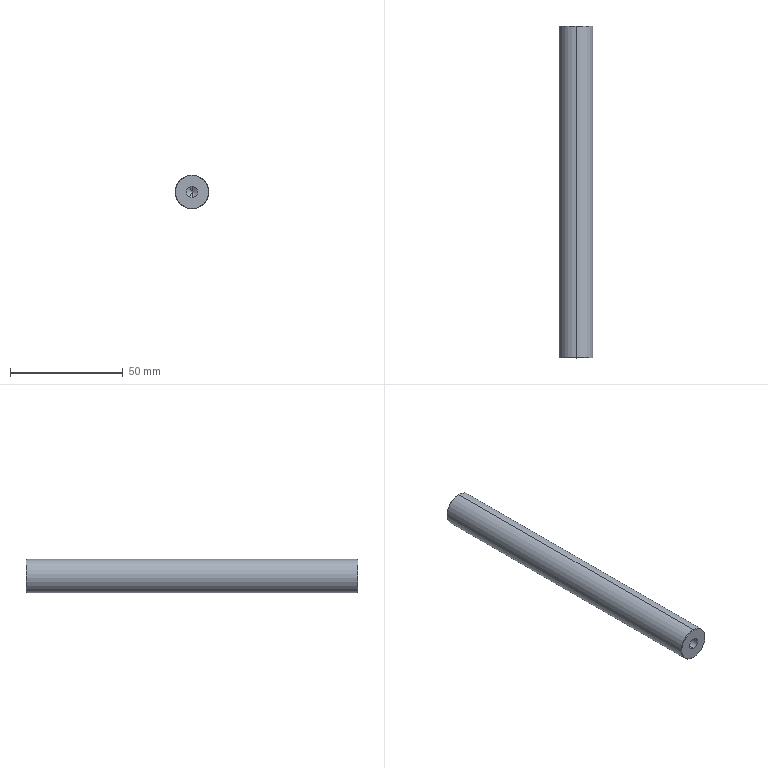Part | STEP file | 1 solid | 16 faces | box 15 x 147 x 15 mm | volume 25052 mm3 | cone 8 | cylinder 6 | plane 2 | commonest cylinder face diameters 5 x4 15 x2
STEP:
#1=CARTESIAN_POINT('',(0.,0.,0.));
#2=DIRECTION('',(0.,0.,1.));
#3=DIRECTION('',(1.,0.,0.));
#4=AXIS2_PLACEMENT_3D('',#1,#2,#3);
#5=CARTESIAN_POINT('',(0.,-73.5,-7.3));
#6=VERTEX_POINT('',#5);
#7=CARTESIAN_POINT('',(0.,-73.5,7.3));
#8=VERTEX_POINT('',#7);
#9=CARTESIAN_POINT('',(0.,-73.5,0.));
#10=DIRECTION('',(0.,-1.,0.));
#11=DIRECTION('',(0.,0.,1.));
#12=AXIS2_PLACEMENT_3D('',#9,#10,#11);
#13=CIRCLE('',#12,7.3);
#14=CARTESIAN_POINT('',(0.,-73.3,0.));
#15=DIRECTION('',(0.,1.,0.));
#16=DIRECTION('',(0.,0.,1.));
#17=AXIS2_PLACEMENT_3D('',#14,#15,#16);
#18=CONICAL_SURFACE('',#17,7.5,0.7854);
#19=CARTESIAN_POINT('',(6.283,-0.2));
#20=DIRECTION('',(-1.,0.));
#21=VECTOR('',#20,1.);
#22=LINE('',#19,#21);
#23=(GEOMETRIC_REPRESENTATION_CONTEXT(2)PARAMETRIC_REPRESENTATION_CONTEXT()REPRESENTATION_CONTEXT('',''));
#24=DEFINITIONAL_REPRESENTATION('',(#22),#23);
#25=PCURVE('',#18,#24);
#26=CARTESIAN_POINT('',(0.,-73.5,0.));
#27=DIRECTION('',(0.,1.,0.));
#28=DIRECTION('',(0.,0.,1.));
#29=AXIS2_PLACEMENT_3D('',#26,#27,#28);
#30=PLANE('',#29);
#31=CARTESIAN_POINT('',(7.3,0.));
#32=CARTESIAN_POINT('',(7.3,-12.644));
#33=CARTESIAN_POINT('',(-3.65,-6.322));
#34=CARTESIAN_POINT('',(-14.6,0.));
#35=CARTESIAN_POINT('',(-3.65,6.322));
#36=CARTESIAN_POINT('',(7.3,12.644));
#37=CARTESIAN_POINT('',(7.3,0.));
#38=(BOUNDED_CURVE()B_SPLINE_CURVE(2,(#31,#32,#33,#34,#35,#36,#37),.UNSPECIFIED.,.T.,.F.)B_SPLINE_CURVE_WITH_KNOTS((1,2,2,2,2,1),(-2.094,0.,2.094,4.189,6.283,8.378),.UNSPECIFIED.)CURVE()GEOMETRIC_REPRESENTATION_ITEM()RATIONAL_B_SPLINE_CURVE((1.,0.5,1.,0.5,1.,0.5,1.))REPRESENTATION_ITEM(''));
#39=(GEOMETRIC_REPRESENTATION_CONTEXT(2)PARAMETRIC_REPRESENTATION_CONTEXT()REPRESENTATION_CONTEXT('',''));
#40=DEFINITIONAL_REPRESENTATION('',(#38),#39);
#41=PCURVE('',#30,#40);
#42=SURFACE_CURVE('',#13,(#25,#41),.PCURVE_S1.);
#43=EDGE_CURVE('',#6,#8,#42,.T.);
#44=ORIENTED_EDGE('',*,*,#43,.F.);
#45=CARTESIAN_POINT('',(0.,-73.3,-7.5));
#46=VERTEX_POINT('',#45);
#47=CARTESIAN_POINT('',(0.,-73.3,-7.5));
#48=DIRECTION('',(0.,0.7071,-0.7071));
#49=VECTOR('',#48,1.);
#50=LINE('',#47,#49);
#51=CARTESIAN_POINT('',(3.142,0.));
#52=DIRECTION('',(0.,1.));
#53=VECTOR('',#52,1.);
#54=LINE('',#51,#53);
#55=(GEOMETRIC_REPRESENTATION_CONTEXT(2)PARAMETRIC_REPRESENTATION_CONTEXT()REPRESENTATION_CONTEXT('',''));
#56=DEFINITIONAL_REPRESENTATION('',(#54),#55);
#57=PCURVE('',#18,#56);
#58=CARTESIAN_POINT('',(0.,-73.3,0.));
#59=DIRECTION('',(0.,1.,0.));
#60=DIRECTION('',(0.,0.,1.));
#61=AXIS2_PLACEMENT_3D('',#58,#59,#60);
#62=CONICAL_SURFACE('',#61,7.5,0.7854);
#63=CARTESIAN_POINT('',(3.142,0.));
#64=DIRECTION('',(0.,1.));
#65=VECTOR('',#64,1.);
#66=LINE('',#63,#65);
#67=(GEOMETRIC_REPRESENTATION_CONTEXT(2)PARAMETRIC_REPRESENTATION_CONTEXT()REPRESENTATION_CONTEXT('',''));
#68=DEFINITIONAL_REPRESENTATION('',(#66),#67);
#69=PCURVE('',#62,#68);
#70=SURFACE_CURVE('',#50,(#57,#69),.PCURVE_S1.);
#71=EDGE_CURVE('',#6,#46,#70,.T.);
#72=ORIENTED_EDGE('',*,*,#71,.T.);
#73=CARTESIAN_POINT('',(0.,-73.3,7.5));
#74=VERTEX_POINT('',#73);
#75=CARTESIAN_POINT('',(0.,-73.3,0.));
#76=DIRECTION('',(0.,1.,0.));
#77=DIRECTION('',(0.,0.,1.));
#78=AXIS2_PLACEMENT_3D('',#75,#76,#77);
#79=CIRCLE('',#78,7.5);
#80=CARTESIAN_POINT('',(0.,0.));
#81=DIRECTION('',(1.,0.));
#82=VECTOR('',#81,1.);
#83=LINE('',#80,#82);
#84=(GEOMETRIC_REPRESENTATION_CONTEXT(2)PARAMETRIC_REPRESENTATION_CONTEXT()REPRESENTATION_CONTEXT('',''));
#85=DEFINITIONAL_REPRESENTATION('',(#83),#84);
#86=PCURVE('',#18,#85);
#87=CARTESIAN_POINT('',(0.,73.5,0.));
#88=DIRECTION('',(0.,-1.,0.));
#89=DIRECTION('',(0.,0.,-1.));
#90=AXIS2_PLACEMENT_3D('',#87,#88,#89);
#91=CYLINDRICAL_SURFACE('',#90,7.5);
#92=CARTESIAN_POINT('',(3.142,146.8));
#93=DIRECTION('',(-1.,0.));
#94=VECTOR('',#93,1.);
#95=LINE('',#92,#94);
#96=(GEOMETRIC_REPRESENTATION_CONTEXT(2)PARAMETRIC_REPRESENTATION_CONTEXT()REPRESENTATION_CONTEXT('',''));
#97=DEFINITIONAL_REPRESENTATION('',(#95),#96);
#98=PCURVE('',#91,#97);
#99=SURFACE_CURVE('',#79,(#86,#98),.PCURVE_S1.);
#100=EDGE_CURVE('',#74,#46,#99,.T.);
#101=ORIENTED_EDGE('',*,*,#100,.F.);
#102=CARTESIAN_POINT('',(0.,-73.3,7.5));
#103=DIRECTION('',(0.,0.7071,0.7071));
#104=VECTOR('',#103,1.);
#105=LINE('',#102,#104);
#106=CARTESIAN_POINT('',(0.,0.));
#107=DIRECTION('',(0.,1.));
#108=VECTOR('',#107,1.);
#109=LINE('',#106,#108);
#110=(GEOMETRIC_REPRESENTATION_CONTEXT(2)PARAMETRIC_REPRESENTATION_CONTEXT()REPRESENTATION_CONTEXT('',''));
#111=DEFINITIONAL_REPRESENTATION('',(#109),#110);
#112=PCURVE('',#18,#111);
#113=CARTESIAN_POINT('',(6.283,0.));
#114=DIRECTION('',(0.,1.));
#115=VECTOR('',#114,1.);
#116=LINE('',#113,#115);
#117=(GEOMETRIC_REPRESENTATION_CONTEXT(2)PARAMETRIC_REPRESENTATION_CONTEXT()REPRESENTATION_CONTEXT('',''));
#118=DEFINITIONAL_REPRESENTATION('',(#116),#117);
#119=PCURVE('',#62,#118);
#120=SURFACE_CURVE('',#105,(#112,#119),.PCURVE_S1.);
#121=EDGE_CURVE('',#8,#74,#120,.T.);
#122=ORIENTED_EDGE('',*,*,#121,.F.);
#123=EDGE_LOOP('',(#44,#72,#101,#122));
#124=FACE_BOUND('',#123,.T.);
#125=ADVANCED_FACE('',(#124),#18,.T.);
#126=CARTESIAN_POINT('',(0.,73.5,7.3));
#127=VERTEX_POINT('',#126);
#128=CARTESIAN_POINT('',(0.,73.5,-7.3));
#129=VERTEX_POINT('',#128);
#130=CARTESIAN_POINT('',(0.,73.5,0.));
#131=DIRECTION('',(0.,1.,0.));
#132=DIRECTION('',(0.,0.,1.));
#133=AXIS2_PLACEMENT_3D('',#130,#131,#132);
#134=CIRCLE('',#133,7.3);
#135=CARTESIAN_POINT('',(0.,73.5,0.));
#136=DIRECTION('',(0.,-1.,0.));
#137=DIRECTION('',(0.,0.,-1.));
#138=AXIS2_PLACEMENT_3D('',#135,#136,#137);
#139=CONICAL_SURFACE('',#138,7.3,0.7854);
#140=CARTESIAN_POINT('',(3.142,0.));
#141=DIRECTION('',(-1.,0.));
#142=VECTOR('',#141,1.);
#143=LINE('',#140,#142);
#144=(GEOMETRIC_REPRESENTATION_CONTEXT(2)PARAMETRIC_REPRESENTATION_CONTEXT()REPRESENTATION_CONTEXT('',''));
#145=DEFINITIONAL_REPRESENTATION('',(#143),#144);
#146=PCURVE('',#139,#145);
#147=CARTESIAN_POINT('',(0.,73.5,0.));
#148=DIRECTION('',(0.,1.,0.));
#149=DIRECTION('',(0.,0.,1.));
#150=AXIS2_PLACEMENT_3D('',#147,#148,#149);
#151=PLANE('',#150);
#152=CARTESIAN_POINT('',(0.,0.));
#153=DIRECTION('',(1.,0.));
#154=AXIS2_PLACEMENT_2D('',#152,#153);
#155=CIRCLE('',#154,7.3);
#156=(GEOMETRIC_REPRESENTATION_CONTEXT(2)PARAMETRIC_REPRESENTATION_CONTEXT()REPRESENTATION_CONTEXT('',''));
#157=DEFINITIONAL_REPRESENTATION('',(#155),#156);
#158=PCURVE('',#151,#157);
#159=SURFACE_CURVE('',#134,(#146,#158),.PCURVE_S1.);
#160=EDGE_CURVE('',#127,#129,#159,.T.);
#161=ORIENTED_EDGE('',*,*,#160,.F.);
#162=CARTESIAN_POINT('',(0.,73.3,7.5));
#163=VERTEX_POINT('',#162);
#164=CARTESIAN_POINT('',(0.,73.5,7.3));
#165=DIRECTION('',(0.,-0.7071,0.7071));
#166=VECTOR('',#165,1.);
#167=LINE('',#164,#166);
#168=CARTESIAN_POINT('',(3.142,0.));
#169=DIRECTION('',(0.,1.));
#170=VECTOR('',#169,1.);
#171=LINE('',#168,#170);
#172=(GEOMETRIC_REPRESENTATION_CONTEXT(2)PARAMETRIC_REPRESENTATION_CONTEXT()REPRESENTATION_CONTEXT('',''));
#173=DEFINITIONAL_REPRESENTATION('',(#171),#172);
#174=PCURVE('',#139,#173);
#175=CARTESIAN_POINT('',(0.,73.5,0.));
#176=DIRECTION('',(0.,-1.,0.));
#177=DIRECTION('',(0.,0.,-1.));
#178=AXIS2_PLACEMENT_3D('',#175,#176,#177);
#179=CONICAL_SURFACE('',#178,7.3,0.7854);
#180=CARTESIAN_POINT('',(3.142,0.));
#181=DIRECTION('',(0.,1.));
#182=VECTOR('',#181,1.);
#183=LINE('',#180,#182);
#184=(GEOMETRIC_REPRESENTATION_CONTEXT(2)PARAMETRIC_REPRESENTATION_CONTEXT()REPRESENTATION_CONTEXT('',''));
#185=DEFINITIONAL_REPRESENTATION('',(#183),#184);
#186=PCURVE('',#179,#185);
#187=SURFACE_CURVE('',#167,(#174,#186),.PCURVE_S1.);
#188=EDGE_CURVE('',#127,#163,#187,.T.);
#189=ORIENTED_EDGE('',*,*,#188,.T.);
#190=CARTESIAN_POINT('',(0.,73.3,-7.5));
#191=VERTEX_POINT('',#190);
#192=CARTESIAN_POINT('',(0.,73.3,0.));
#193=DIRECTION('',(0.,-1.,0.));
#194=DIRECTION('',(0.,0.,1.));
#195=AXIS2_PLACEMENT_3D('',#192,#193,#194);
#196=CIRCLE('',#195,7.5);
#197=CARTESIAN_POINT('',(-3.142,0.2));
#198=DIRECTION('',(1.,0.));
#199=VECTOR('',#198,1.);
#200=LINE('',#197,#199);
#201=(GEOMETRIC_REPRESENTATION_CONTEXT(2)PARAMETRIC_REPRESENTATION_CONTEXT()REPRESENTATION_CONTEXT('',''));
#202=DEFINITIONAL_REPRESENTATION('',(#200),#201);
#203=PCURVE('',#139,#202);
#204=CARTESIAN_POINT('',(-3.142,0.2));
#205=DIRECTION('',(1.,0.));
#206=VECTOR('',#205,1.);
#207=LINE('',#204,#206);
#208=(GEOMETRIC_REPRESENTATION_CONTEXT(2)PARAMETRIC_REPRESENTATION_CONTEXT()REPRESENTATION_CONTEXT('',''));
#209=DEFINITIONAL_REPRESENTATION('',(#207),#208);
#210=PCURVE('',#91,#209);
#211=SURFACE_CURVE('',#196,(#203,#210),.PCURVE_S1.);
#212=EDGE_CURVE('',#191,#163,#211,.T.);
#213=ORIENTED_EDGE('',*,*,#212,.F.);
#214=CARTESIAN_POINT('',(0.,73.5,-7.3));
#215=DIRECTION('',(0.,-0.7071,-0.7071));
#216=VECTOR('',#215,1.);
#217=LINE('',#214,#216);
#218=CARTESIAN_POINT('',(0.,0.));
#219=DIRECTION('',(0.,1.));
#220=VECTOR('',#219,1.);
#221=LINE('',#218,#220);
#222=(GEOMETRIC_REPRESENTATION_CONTEXT(2)PARAMETRIC_REPRESENTATION_CONTEXT()REPRESENTATION_CONTEXT('',''));
#223=DEFINITIONAL_REPRESENTATION('',(#221),#222);
#224=PCURVE('',#139,#223);
#225=CARTESIAN_POINT('',(6.283,0.));
#226=DIRECTION('',(0.,1.));
#227=VECTOR('',#226,1.);
#228=LINE('',#225,#227);
#229=(GEOMETRIC_REPRESENTATION_CONTEXT(2)PARAMETRIC_REPRESENTATION_CONTEXT()REPRESENTATION_CONTEXT('',''));
#230=DEFINITIONAL_REPRESENTATION('',(#228),#229);
#231=PCURVE('',#179,#230);
#232=SURFACE_CURVE('',#217,(#224,#231),.PCURVE_S1.);
#233=EDGE_CURVE('',#129,#191,#232,.T.);
#234=ORIENTED_EDGE('',*,*,#233,.F.);
#235=EDGE_LOOP('',(#161,#189,#213,#234));
#236=FACE_BOUND('',#235,.T.);
#237=ADVANCED_FACE('',(#236),#139,.T.);
#238=CARTESIAN_POINT('',(0.,-50.5,-2.5));
#239=VERTEX_POINT('',#238);
#240=CARTESIAN_POINT('',(0.,-73.5,-2.5));
#241=VERTEX_POINT('',#240);
#242=CARTESIAN_POINT('',(0.,-73.5,-2.5));
#243=DIRECTION('',(0.,-1.,0.));
#244=VECTOR('',#243,1.);
#245=LINE('',#242,#244);
#246=CARTESIAN_POINT('',(0.,-73.5,0.));
#247=DIRECTION('',(0.,-1.,0.));
#248=DIRECTION('',(0.,0.,-1.));
#249=AXIS2_PLACEMENT_3D('',#246,#247,#248);
#250=CYLINDRICAL_SURFACE('',#249,2.5);
#251=CARTESIAN_POINT('',(6.283,0.));
#252=DIRECTION('',(0.,1.));
#253=VECTOR('',#252,1.);
#254=LINE('',#251,#253);
#255=(GEOMETRIC_REPRESENTATION_CONTEXT(2)PARAMETRIC_REPRESENTATION_CONTEXT()REPRESENTATION_CONTEXT('',''));
#256=DEFINITIONAL_REPRESENTATION('',(#254),#255);
#257=PCURVE('',#250,#256);
#258=CARTESIAN_POINT('',(0.,-73.5,0.));
#259=DIRECTION('',(0.,-1.,0.));
#260=DIRECTION('',(0.,0.,-1.));
#261=AXIS2_PLACEMENT_3D('',#258,#259,#260);
#262=CYLINDRICAL_SURFACE('',#261,2.5);
#263=CARTESIAN_POINT('',(0.,0.));
#264=DIRECTION('',(0.,1.));
#265=VECTOR('',#264,1.);
#266=LINE('',#263,#265);
#267=(GEOMETRIC_REPRESENTATION_CONTEXT(2)PARAMETRIC_REPRESENTATION_CONTEXT()REPRESENTATION_CONTEXT('',''));
#268=DEFINITIONAL_REPRESENTATION('',(#266),#267);
#269=PCURVE('',#262,#268);
#270=SURFACE_CURVE('',#245,(#257,#269),.PCURVE_S1.);
#271=EDGE_CURVE('',#239,#241,#270,.T.);
#272=ORIENTED_EDGE('',*,*,#271,.T.);
#273=CARTESIAN_POINT('',(0.,-73.5,2.5));
#274=VERTEX_POINT('',#273);
#275=CARTESIAN_POINT('',(0.,-73.5,0.));
#276=DIRECTION('',(0.,-1.,0.));
#277=DIRECTION('',(0.,0.,-1.));
#278=AXIS2_PLACEMENT_3D('',#275,#276,#277);
#279=CIRCLE('',#278,2.5);
#280=CARTESIAN_POINT('',(0.,0.));
#281=DIRECTION('',(1.,0.));
#282=VECTOR('',#281,1.);
#283=LINE('',#280,#282);
#284=(GEOMETRIC_REPRESENTATION_CONTEXT(2)PARAMETRIC_REPRESENTATION_CONTEXT()REPRESENTATION_CONTEXT('',''));
#285=DEFINITIONAL_REPRESENTATION('',(#283),#284);
#286=PCURVE('',#250,#285);
#287=CARTESIAN_POINT('',(-2.5,0.));
#288=CARTESIAN_POINT('',(-2.5,4.33));
#289=CARTESIAN_POINT('',(1.25,2.165));
#290=CARTESIAN_POINT('',(5.,0.));
#291=CARTESIAN_POINT('',(1.25,-2.165));
#292=CARTESIAN_POINT('',(-2.5,-4.33));
#293=CARTESIAN_POINT('',(-2.5,0.));
#294=(BOUNDED_CURVE()B_SPLINE_CURVE(2,(#287,#288,#289,#290,#291,#292,#293),.UNSPECIFIED.,.T.,.F.)B_SPLINE_CURVE_WITH_KNOTS((1,2,2,2,2,1),(-2.094,0.,2.094,4.189,6.283,8.378),.UNSPECIFIED.)CURVE()GEOMETRIC_REPRESENTATION_ITEM()RATIONAL_B_SPLINE_CURVE((1.,0.5,1.,0.5,1.,0.5,1.))REPRESENTATION_ITEM(''));
#295=(GEOMETRIC_REPRESENTATION_CONTEXT(2)PARAMETRIC_REPRESENTATION_CONTEXT()REPRESENTATION_CONTEXT('',''));
#296=DEFINITIONAL_REPRESENTATION('',(#294),#295);
#297=PCURVE('',#30,#296);
#298=SURFACE_CURVE('',#279,(#286,#297),.PCURVE_S1.);
#299=EDGE_CURVE('',#274,#241,#298,.T.);
#300=ORIENTED_EDGE('',*,*,#299,.F.);
#301=CARTESIAN_POINT('',(0.,-50.5,2.5));
#302=VERTEX_POINT('',#301);
#303=CARTESIAN_POINT('',(0.,-73.5,2.5));
#304=DIRECTION('',(0.,-1.,0.));
#305=VECTOR('',#304,1.);
#306=LINE('',#303,#305);
#307=CARTESIAN_POINT('',(3.142,0.));
#308=DIRECTION('',(0.,1.));
#309=VECTOR('',#308,1.);
#310=LINE('',#307,#309);
#311=(GEOMETRIC_REPRESENTATION_CONTEXT(2)PARAMETRIC_REPRESENTATION_CONTEXT()REPRESENTATION_CONTEXT('',''));
#312=DEFINITIONAL_REPRESENTATION('',(#310),#311);
#313=PCURVE('',#250,#312);
#314=CARTESIAN_POINT('',(3.142,0.));
#315=DIRECTION('',(0.,1.));
#316=VECTOR('',#315,1.);
#317=LINE('',#314,#316);
#318=(GEOMETRIC_REPRESENTATION_CONTEXT(2)PARAMETRIC_REPRESENTATION_CONTEXT()REPRESENTATION_CONTEXT('',''));
#319=DEFINITIONAL_REPRESENTATION('',(#317),#318);
#320=PCURVE('',#262,#319);
#321=SURFACE_CURVE('',#306,(#313,#320),.PCURVE_S1.);
#322=EDGE_CURVE('',#302,#274,#321,.T.);
#323=ORIENTED_EDGE('',*,*,#322,.F.);
#324=CARTESIAN_POINT('',(0.,-50.5,0.));
#325=DIRECTION('',(0.,-1.,0.));
#326=DIRECTION('',(0.,0.,-1.));
#327=AXIS2_PLACEMENT_3D('',#324,#325,#326);
#328=CIRCLE('',#327,2.5);
#329=CARTESIAN_POINT('',(0.,-23.));
#330=DIRECTION('',(1.,0.));
#331=VECTOR('',#330,1.);
#332=LINE('',#329,#331);
#333=(GEOMETRIC_REPRESENTATION_CONTEXT(2)PARAMETRIC_REPRESENTATION_CONTEXT()REPRESENTATION_CONTEXT('',''));
#334=DEFINITIONAL_REPRESENTATION('',(#332),#333);
#335=PCURVE('',#250,#334);
#336=CARTESIAN_POINT('',(0.,-50.5,0.));
#337=DIRECTION('',(0.,-1.,0.));
#338=DIRECTION('',(0.,0.,-1.));
#339=AXIS2_PLACEMENT_3D('',#336,#337,#338);
#340=CONICAL_SURFACE('',#339,2.5,1.03);
#341=CARTESIAN_POINT('',(0.,0.));
#342=DIRECTION('',(1.,0.));
#343=VECTOR('',#342,1.);
#344=LINE('',#341,#343);
#345=(GEOMETRIC_REPRESENTATION_CONTEXT(2)PARAMETRIC_REPRESENTATION_CONTEXT()REPRESENTATION_CONTEXT('',''));
#346=DEFINITIONAL_REPRESENTATION('',(#344),#345);
#347=PCURVE('',#340,#346);
#348=SURFACE_CURVE('',#328,(#335,#347),.PCURVE_S1.);
#349=EDGE_CURVE('',#302,#239,#348,.T.);
#350=ORIENTED_EDGE('',*,*,#349,.T.);
#351=EDGE_LOOP('',(#272,#300,#323,#350));
#352=FACE_BOUND('',#351,.F.);
#353=ADVANCED_FACE('',(#352),#250,.F.);
#354=ORIENTED_EDGE('',*,*,#349,.F.);
#355=CARTESIAN_POINT('',(0.,-48.998,0.));
#356=VERTEX_POINT('',#355);
#357=CARTESIAN_POINT('',(0.,-50.5,2.5));
#358=DIRECTION('',(0.,-0.515,0.8572));
#359=VECTOR('',#358,1.);
#360=LINE('',#357,#359);
#361=CARTESIAN_POINT('',(3.142,0.));
#362=DIRECTION('',(0.,1.));
#363=VECTOR('',#362,1.);
#364=LINE('',#361,#363);
#365=(GEOMETRIC_REPRESENTATION_CONTEXT(2)PARAMETRIC_REPRESENTATION_CONTEXT()REPRESENTATION_CONTEXT('',''));
#366=DEFINITIONAL_REPRESENTATION('',(#364),#365);
#367=PCURVE('',#340,#366);
#368=CARTESIAN_POINT('',(0.,-50.5,0.));
#369=DIRECTION('',(0.,-1.,0.));
#370=DIRECTION('',(0.,0.,-1.));
#371=AXIS2_PLACEMENT_3D('',#368,#369,#370);
#372=CONICAL_SURFACE('',#371,2.5,1.03);
#373=CARTESIAN_POINT('',(3.142,0.));
#374=DIRECTION('',(0.,1.));
#375=VECTOR('',#374,1.);
#376=LINE('',#373,#375);
#377=(GEOMETRIC_REPRESENTATION_CONTEXT(2)PARAMETRIC_REPRESENTATION_CONTEXT()REPRESENTATION_CONTEXT('',''));
#378=DEFINITIONAL_REPRESENTATION('',(#376),#377);
#379=PCURVE('',#372,#378);
#380=SURFACE_CURVE('',#360,(#367,#379),.PCURVE_S1.);
#381=EDGE_CURVE('',#356,#302,#380,.T.);
#382=ORIENTED_EDGE('',*,*,#381,.F.);
#383=CARTESIAN_POINT('',(0.,-50.5,-2.5));
#384=DIRECTION('',(0.,-0.515,-0.8572));
#385=VECTOR('',#384,1.);
#386=LINE('',#383,#385);
#387=CARTESIAN_POINT('',(6.283,0.));
#388=DIRECTION('',(0.,1.));
#389=VECTOR('',#388,1.);
#390=LINE('',#387,#389);
#391=(GEOMETRIC_REPRESENTATION_CONTEXT(2)PARAMETRIC_REPRESENTATION_CONTEXT()REPRESENTATION_CONTEXT('',''));
#392=DEFINITIONAL_REPRESENTATION('',(#390),#391);
#393=PCURVE('',#340,#392);
#394=CARTESIAN_POINT('',(0.,0.));
#395=DIRECTION('',(0.,1.));
#396=VECTOR('',#395,1.);
#397=LINE('',#394,#396);
#398=(GEOMETRIC_REPRESENTATION_CONTEXT(2)PARAMETRIC_REPRESENTATION_CONTEXT()REPRESENTATION_CONTEXT('',''));
#399=DEFINITIONAL_REPRESENTATION('',(#397),#398);
#400=PCURVE('',#372,#399);
#401=SURFACE_CURVE('',#386,(#393,#400),.PCURVE_S1.);
#402=EDGE_CURVE('',#356,#239,#401,.T.);
#403=ORIENTED_EDGE('',*,*,#402,.T.);
#404=EDGE_LOOP('',(#354,#382,#403));
#405=FACE_BOUND('',#404,.F.);
#406=ADVANCED_FACE('',(#405),#340,.F.);
#407=CARTESIAN_POINT('',(0.,50.5,2.5));
#408=VERTEX_POINT('',#407);
#409=CARTESIAN_POINT('',(0.,73.5,2.5));
#410=VERTEX_POINT('',#409);
#411=CARTESIAN_POINT('',(0.,73.5,2.5));
#412=DIRECTION('',(0.,1.,0.));
#413=VECTOR('',#412,1.);
#414=LINE('',#411,#413);
#415=CARTESIAN_POINT('',(0.,73.5,0.));
#416=DIRECTION('',(0.,1.,0.));
#417=DIRECTION('',(0.,0.,1.));
#418=AXIS2_PLACEMENT_3D('',#415,#416,#417);
#419=CYLINDRICAL_SURFACE('',#418,2.5);
#420=CARTESIAN_POINT('',(6.283,0.));
#421=DIRECTION('',(0.,1.));
#422=VECTOR('',#421,1.);
#423=LINE('',#420,#422);
#424=(GEOMETRIC_REPRESENTATION_CONTEXT(2)PARAMETRIC_REPRESENTATION_CONTEXT()REPRESENTATION_CONTEXT('',''));
#425=DEFINITIONAL_REPRESENTATION('',(#423),#424);
#426=PCURVE('',#419,#425);
#427=CARTESIAN_POINT('',(0.,73.5,0.));
#428=DIRECTION('',(0.,1.,0.));
#429=DIRECTION('',(0.,0.,1.));
#430=AXIS2_PLACEMENT_3D('',#427,#428,#429);
#431=CYLINDRICAL_SURFACE('',#430,2.5);
#432=CARTESIAN_POINT('',(0.,0.));
#433=DIRECTION('',(0.,1.));
#434=VECTOR('',#433,1.);
#435=LINE('',#432,#434);
#436=(GEOMETRIC_REPRESENTATION_CONTEXT(2)PARAMETRIC_REPRESENTATION_CONTEXT()REPRESENTATION_CONTEXT('',''));
#437=DEFINITIONAL_REPRESENTATION('',(#435),#436);
#438=PCURVE('',#431,#437);
#439=SURFACE_CURVE('',#414,(#426,#438),.PCURVE_S1.);
#440=EDGE_CURVE('',#408,#410,#439,.T.);
#441=ORIENTED_EDGE('',*,*,#440,.T.);
#442=CARTESIAN_POINT('',(0.,73.5,-2.5));
#443=VERTEX_POINT('',#442);
#444=CARTESIAN_POINT('',(0.,73.5,0.));
#445=DIRECTION('',(0.,1.,0.));
#446=DIRECTION('',(0.,0.,1.));
#447=AXIS2_PLACEMENT_3D('',#444,#445,#446);
#448=CIRCLE('',#447,2.5);
#449=CARTESIAN_POINT('',(0.,0.));
#450=DIRECTION('',(1.,0.));
#451=VECTOR('',#450,1.);
#452=LINE('',#449,#451);
#453=(GEOMETRIC_REPRESENTATION_CONTEXT(2)PARAMETRIC_REPRESENTATION_CONTEXT()REPRESENTATION_CONTEXT('',''));
#454=DEFINITIONAL_REPRESENTATION('',(#452),#453);
#455=PCURVE('',#419,#454);
#456=CARTESIAN_POINT('',(0.,0.));
#457=DIRECTION('',(1.,0.));
#458=AXIS2_PLACEMENT_2D('',#456,#457);
#459=CIRCLE('',#458,2.5);
#460=(GEOMETRIC_REPRESENTATION_CONTEXT(2)PARAMETRIC_REPRESENTATION_CONTEXT()REPRESENTATION_CONTEXT('',''));
#461=DEFINITIONAL_REPRESENTATION('',(#459),#460);
#462=PCURVE('',#151,#461);
#463=SURFACE_CURVE('',#448,(#455,#462),.PCURVE_S1.);
#464=EDGE_CURVE('',#443,#410,#463,.T.);
#465=ORIENTED_EDGE('',*,*,#464,.F.);
#466=CARTESIAN_POINT('',(0.,50.5,-2.5));
#467=VERTEX_POINT('',#466);
#468=CARTESIAN_POINT('',(0.,73.5,-2.5));
#469=DIRECTION('',(0.,1.,0.));
#470=VECTOR('',#469,1.);
#471=LINE('',#468,#470);
#472=CARTESIAN_POINT('',(3.142,0.));
#473=DIRECTION('',(0.,1.));
#474=VECTOR('',#473,1.);
#475=LINE('',#472,#474);
#476=(GEOMETRIC_REPRESENTATION_CONTEXT(2)PARAMETRIC_REPRESENTATION_CONTEXT()REPRESENTATION_CONTEXT('',''));
#477=DEFINITIONAL_REPRESENTATION('',(#475),#476);
#478=PCURVE('',#419,#477);
#479=CARTESIAN_POINT('',(3.142,0.));
#480=DIRECTION('',(0.,1.));
#481=VECTOR('',#480,1.);
#482=LINE('',#479,#481);
#483=(GEOMETRIC_REPRESENTATION_CONTEXT(2)PARAMETRIC_REPRESENTATION_CONTEXT()REPRESENTATION_CONTEXT('',''));
#484=DEFINITIONAL_REPRESENTATION('',(#482),#483);
#485=PCURVE('',#431,#484);
#486=SURFACE_CURVE('',#471,(#478,#485),.PCURVE_S1.);
#487=EDGE_CURVE('',#467,#443,#486,.T.);
#488=ORIENTED_EDGE('',*,*,#487,.F.);
#489=CARTESIAN_POINT('',(0.,50.5,0.));
#490=DIRECTION('',(0.,1.,0.));
#491=DIRECTION('',(0.,0.,1.));
#492=AXIS2_PLACEMENT_3D('',#489,#490,#491);
#493=CIRCLE('',#492,2.5);
#494=CARTESIAN_POINT('',(0.,-23.));
#495=DIRECTION('',(1.,0.));
#496=VECTOR('',#495,1.);
#497=LINE('',#494,#496);
#498=(GEOMETRIC_REPRESENTATION_CONTEXT(2)PARAMETRIC_REPRESENTATION_CONTEXT()REPRESENTATION_CONTEXT('',''));
#499=DEFINITIONAL_REPRESENTATION('',(#497),#498);
#500=PCURVE('',#419,#499);
#501=CARTESIAN_POINT('',(0.,50.5,0.));
#502=DIRECTION('',(0.,1.,0.));
#503=DIRECTION('',(0.,0.,1.));
#504=AXIS2_PLACEMENT_3D('',#501,#502,#503);
#505=CONICAL_SURFACE('',#504,2.5,1.03);
#506=CARTESIAN_POINT('',(0.,0.));
#507=DIRECTION('',(1.,0.));
#508=VECTOR('',#507,1.);
#509=LINE('',#506,#508);
#510=(GEOMETRIC_REPRESENTATION_CONTEXT(2)PARAMETRIC_REPRESENTATION_CONTEXT()REPRESENTATION_CONTEXT('',''));
#511=DEFINITIONAL_REPRESENTATION('',(#509),#510);
#512=PCURVE('',#505,#511);
#513=SURFACE_CURVE('',#493,(#500,#512),.PCURVE_S1.);
#514=EDGE_CURVE('',#467,#408,#513,.T.);
#515=ORIENTED_EDGE('',*,*,#514,.T.);
#516=EDGE_LOOP('',(#441,#465,#488,#515));
#517=FACE_BOUND('',#516,.F.);
#518=ADVANCED_FACE('',(#517),#419,.F.);
#519=ORIENTED_EDGE('',*,*,#514,.F.);
#520=CARTESIAN_POINT('',(0.,48.998,0.));
#521=VERTEX_POINT('',#520);
#522=CARTESIAN_POINT('',(0.,50.5,-2.5));
#523=DIRECTION('',(0.,0.515,-0.8572));
#524=VECTOR('',#523,1.);
#525=LINE('',#522,#524);
#526=CARTESIAN_POINT('',(3.142,0.));
#527=DIRECTION('',(0.,1.));
#528=VECTOR('',#527,1.);
#529=LINE('',#526,#528);
#530=(GEOMETRIC_REPRESENTATION_CONTEXT(2)PARAMETRIC_REPRESENTATION_CONTEXT()REPRESENTATION_CONTEXT('',''));
#531=DEFINITIONAL_REPRESENTATION('',(#529),#530);
#532=PCURVE('',#505,#531);
#533=CARTESIAN_POINT('',(0.,50.5,0.));
#534=DIRECTION('',(0.,1.,0.));
#535=DIRECTION('',(0.,0.,1.));
#536=AXIS2_PLACEMENT_3D('',#533,#534,#535);
#537=CONICAL_SURFACE('',#536,2.5,1.03);
#538=CARTESIAN_POINT('',(3.142,0.));
#539=DIRECTION('',(0.,1.));
#540=VECTOR('',#539,1.);
#541=LINE('',#538,#540);
#542=(GEOMETRIC_REPRESENTATION_CONTEXT(2)PARAMETRIC_REPRESENTATION_CONTEXT()REPRESENTATION_CONTEXT('',''));
#543=DEFINITIONAL_REPRESENTATION('',(#541),#542);
#544=PCURVE('',#537,#543);
#545=SURFACE_CURVE('',#525,(#532,#544),.PCURVE_S1.);
#546=EDGE_CURVE('',#521,#467,#545,.T.);
#547=ORIENTED_EDGE('',*,*,#546,.F.);
#548=CARTESIAN_POINT('',(0.,50.5,2.5));
#549=DIRECTION('',(0.,0.515,0.8572));
#550=VECTOR('',#549,1.);
#551=LINE('',#548,#550);
#552=CARTESIAN_POINT('',(6.283,0.));
#553=DIRECTION('',(0.,1.));
#554=VECTOR('',#553,1.);
#555=LINE('',#552,#554);
#556=(GEOMETRIC_REPRESENTATION_CONTEXT(2)PARAMETRIC_REPRESENTATION_CONTEXT()REPRESENTATION_CONTEXT('',''));
#557=DEFINITIONAL_REPRESENTATION('',(#555),#556);
#558=PCURVE('',#505,#557);
#559=CARTESIAN_POINT('',(0.,0.));
#560=DIRECTION('',(0.,1.));
#561=VECTOR('',#560,1.);
#562=LINE('',#559,#561);
#563=(GEOMETRIC_REPRESENTATION_CONTEXT(2)PARAMETRIC_REPRESENTATION_CONTEXT()REPRESENTATION_CONTEXT('',''));
#564=DEFINITIONAL_REPRESENTATION('',(#562),#563);
#565=PCURVE('',#537,#564);
#566=SURFACE_CURVE('',#551,(#558,#565),.PCURVE_S1.);
#567=EDGE_CURVE('',#521,#408,#566,.T.);
#568=ORIENTED_EDGE('',*,*,#567,.T.);
#569=EDGE_LOOP('',(#519,#547,#568));
#570=FACE_BOUND('',#569,.F.);
#571=ADVANCED_FACE('',(#570),#505,.F.);
#572=ORIENTED_EDGE('',*,*,#212,.T.);
#573=CARTESIAN_POINT('',(0.,73.5,7.5));
#574=DIRECTION('',(0.,-1.,0.));
#575=VECTOR('',#574,1.);
#576=LINE('',#573,#575);
#577=CARTESIAN_POINT('',(3.142,0.));
#578=DIRECTION('',(0.,1.));
#579=VECTOR('',#578,1.);
#580=LINE('',#577,#579);
#581=(GEOMETRIC_REPRESENTATION_CONTEXT(2)PARAMETRIC_REPRESENTATION_CONTEXT()REPRESENTATION_CONTEXT('',''));
#582=DEFINITIONAL_REPRESENTATION('',(#580),#581);
#583=PCURVE('',#91,#582);
#584=CARTESIAN_POINT('',(0.,73.5,0.));
#585=DIRECTION('',(0.,-1.,0.));
#586=DIRECTION('',(0.,0.,-1.));
#587=AXIS2_PLACEMENT_3D('',#584,#585,#586);
#588=CYLINDRICAL_SURFACE('',#587,7.5);
#589=CARTESIAN_POINT('',(3.142,0.));
#590=DIRECTION('',(0.,1.));
#591=VECTOR('',#590,1.);
#592=LINE('',#589,#591);
#593=(GEOMETRIC_REPRESENTATION_CONTEXT(2)PARAMETRIC_REPRESENTATION_CONTEXT()REPRESENTATION_CONTEXT('',''));
#594=DEFINITIONAL_REPRESENTATION('',(#592),#593);
#595=PCURVE('',#588,#594);
#596=SURFACE_CURVE('',#576,(#583,#595),.PCURVE_S1.);
#597=EDGE_CURVE('',#163,#74,#596,.T.);
#598=ORIENTED_EDGE('',*,*,#597,.T.);
#599=ORIENTED_EDGE('',*,*,#100,.T.);
#600=CARTESIAN_POINT('',(0.,73.5,-7.5));
#601=DIRECTION('',(0.,-1.,0.));
#602=VECTOR('',#601,1.);
#603=LINE('',#600,#602);
#604=CARTESIAN_POINT('',(0.,0.));
#605=DIRECTION('',(0.,1.));
#606=VECTOR('',#605,1.);
#607=LINE('',#604,#606);
#608=(GEOMETRIC_REPRESENTATION_CONTEXT(2)PARAMETRIC_REPRESENTATION_CONTEXT()REPRESENTATION_CONTEXT('',''));
#609=DEFINITIONAL_REPRESENTATION('',(#607),#608);
#610=PCURVE('',#91,#609);
#611=CARTESIAN_POINT('',(6.283,0.));
#612=DIRECTION('',(0.,1.));
#613=VECTOR('',#612,1.);
#614=LINE('',#611,#613);
#615=(GEOMETRIC_REPRESENTATION_CONTEXT(2)PARAMETRIC_REPRESENTATION_CONTEXT()REPRESENTATION_CONTEXT('',''));
#616=DEFINITIONAL_REPRESENTATION('',(#614),#615);
#617=PCURVE('',#588,#616);
#618=SURFACE_CURVE('',#603,(#610,#617),.PCURVE_S1.);
#619=EDGE_CURVE('',#191,#46,#618,.T.);
#620=ORIENTED_EDGE('',*,*,#619,.F.);
#621=EDGE_LOOP('',(#572,#598,#599,#620));
#622=FACE_BOUND('',#621,.T.);
#623=ADVANCED_FACE('',(#622),#91,.T.);
#624=ORIENTED_EDGE('',*,*,#597,.F.);
#625=CARTESIAN_POINT('',(0.,73.3,0.));
#626=DIRECTION('',(0.,-1.,0.));
#627=DIRECTION('',(0.,0.,1.));
#628=AXIS2_PLACEMENT_3D('',#625,#626,#627);
#629=CIRCLE('',#628,7.5);
#630=CARTESIAN_POINT('',(3.142,0.2));
#631=DIRECTION('',(1.,0.));
#632=VECTOR('',#631,1.);
#633=LINE('',#630,#632);
#634=(GEOMETRIC_REPRESENTATION_CONTEXT(2)PARAMETRIC_REPRESENTATION_CONTEXT()REPRESENTATION_CONTEXT('',''));
#635=DEFINITIONAL_REPRESENTATION('',(#633),#634);
#636=PCURVE('',#588,#635);
#637=CARTESIAN_POINT('',(3.142,0.2));
#638=DIRECTION('',(1.,0.));
#639=VECTOR('',#638,1.);
#640=LINE('',#637,#639);
#641=(GEOMETRIC_REPRESENTATION_CONTEXT(2)PARAMETRIC_REPRESENTATION_CONTEXT()REPRESENTATION_CONTEXT('',''));
#642=DEFINITIONAL_REPRESENTATION('',(#640),#641);
#643=PCURVE('',#179,#642);
#644=SURFACE_CURVE('',#629,(#636,#643),.PCURVE_S1.);
#645=EDGE_CURVE('',#163,#191,#644,.T.);
#646=ORIENTED_EDGE('',*,*,#645,.T.);
#647=ORIENTED_EDGE('',*,*,#619,.T.);
#648=CARTESIAN_POINT('',(0.,-73.3,0.));
#649=DIRECTION('',(0.,1.,0.));
#650=DIRECTION('',(0.,0.,1.));
#651=AXIS2_PLACEMENT_3D('',#648,#649,#650);
#652=CIRCLE('',#651,7.5);
#653=CARTESIAN_POINT('',(9.425,146.8));
#654=DIRECTION('',(-1.,0.));
#655=VECTOR('',#654,1.);
#656=LINE('',#653,#655);
#657=(GEOMETRIC_REPRESENTATION_CONTEXT(2)PARAMETRIC_REPRESENTATION_CONTEXT()REPRESENTATION_CONTEXT('',''));
#658=DEFINITIONAL_REPRESENTATION('',(#656),#657);
#659=PCURVE('',#588,#658);
#660=CARTESIAN_POINT('',(0.,0.));
#661=DIRECTION('',(1.,0.));
#662=VECTOR('',#661,1.);
#663=LINE('',#660,#662);
#664=(GEOMETRIC_REPRESENTATION_CONTEXT(2)PARAMETRIC_REPRESENTATION_CONTEXT()REPRESENTATION_CONTEXT('',''));
#665=DEFINITIONAL_REPRESENTATION('',(#663),#664);
#666=PCURVE('',#62,#665);
#667=SURFACE_CURVE('',#652,(#659,#666),.PCURVE_S1.);
#668=EDGE_CURVE('',#46,#74,#667,.T.);
#669=ORIENTED_EDGE('',*,*,#668,.T.);
#670=EDGE_LOOP('',(#624,#646,#647,#669));
#671=FACE_BOUND('',#670,.T.);
#672=ADVANCED_FACE('',(#671),#588,.T.);
#673=CARTESIAN_POINT('',(0.,73.5,0.));
#674=DIRECTION('',(0.,1.,0.));
#675=DIRECTION('',(0.,0.,1.));
#676=AXIS2_PLACEMENT_3D('',#673,#674,#675);
#677=CIRCLE('',#676,7.3);
#678=CARTESIAN_POINT('',(0.,0.));
#679=DIRECTION('',(1.,0.));
#680=AXIS2_PLACEMENT_2D('',#678,#679);
#681=CIRCLE('',#680,7.3);
#682=(GEOMETRIC_REPRESENTATION_CONTEXT(2)PARAMETRIC_REPRESENTATION_CONTEXT()REPRESENTATION_CONTEXT('',''));
#683=DEFINITIONAL_REPRESENTATION('',(#681),#682);
#684=PCURVE('',#151,#683);
#685=CARTESIAN_POINT('',(9.425,0.));
#686=DIRECTION('',(-1.,0.));
#687=VECTOR('',#686,1.);
#688=LINE('',#685,#687);
#689=(GEOMETRIC_REPRESENTATION_CONTEXT(2)PARAMETRIC_REPRESENTATION_CONTEXT()REPRESENTATION_CONTEXT('',''));
#690=DEFINITIONAL_REPRESENTATION('',(#688),#689);
#691=PCURVE('',#179,#690);
#692=SURFACE_CURVE('',#677,(#684,#691),.PCURVE_S1.);
#693=EDGE_CURVE('',#129,#127,#692,.T.);
#694=ORIENTED_EDGE('',*,*,#693,.T.);
#695=ORIENTED_EDGE('',*,*,#160,.T.);
#696=EDGE_LOOP('',(#694,#695));
#697=FACE_BOUND('',#696,.T.);
#698=CARTESIAN_POINT('',(0.,73.5,0.));
#699=DIRECTION('',(0.,1.,0.));
#700=DIRECTION('',(0.,0.,1.));
#701=AXIS2_PLACEMENT_3D('',#698,#699,#700);
#702=CIRCLE('',#701,2.5);
#703=CARTESIAN_POINT('',(0.,0.));
#704=DIRECTION('',(1.,0.));
#705=AXIS2_PLACEMENT_2D('',#703,#704);
#706=CIRCLE('',#705,2.5);
#707=(GEOMETRIC_REPRESENTATION_CONTEXT(2)PARAMETRIC_REPRESENTATION_CONTEXT()REPRESENTATION_CONTEXT('',''));
#708=DEFINITIONAL_REPRESENTATION('',(#706),#707);
#709=PCURVE('',#151,#708);
#710=CARTESIAN_POINT('',(0.,0.));
#711=DIRECTION('',(1.,0.));
#712=VECTOR('',#711,1.);
#713=LINE('',#710,#712);
#714=(GEOMETRIC_REPRESENTATION_CONTEXT(2)PARAMETRIC_REPRESENTATION_CONTEXT()REPRESENTATION_CONTEXT('',''));
#715=DEFINITIONAL_REPRESENTATION('',(#713),#714);
#716=PCURVE('',#431,#715);
#717=SURFACE_CURVE('',#702,(#709,#716),.PCURVE_S1.);
#718=EDGE_CURVE('',#410,#443,#717,.T.);
#719=ORIENTED_EDGE('',*,*,#718,.F.);
#720=ORIENTED_EDGE('',*,*,#464,.F.);
#721=EDGE_LOOP('',(#719,#720));
#722=FACE_BOUND('',#721,.T.);
#723=ADVANCED_FACE('',(#697,#722),#151,.T.);
#724=CARTESIAN_POINT('',(0.,-73.5,0.));
#725=DIRECTION('',(0.,-1.,0.));
#726=DIRECTION('',(0.,0.,1.));
#727=AXIS2_PLACEMENT_3D('',#724,#725,#726);
#728=CIRCLE('',#727,7.3);
#729=CARTESIAN_POINT('',(7.3,0.));
#730=CARTESIAN_POINT('',(7.3,-12.644));
#731=CARTESIAN_POINT('',(-3.65,-6.322));
#732=CARTESIAN_POINT('',(-14.6,0.));
#733=CARTESIAN_POINT('',(-3.65,6.322));
#734=CARTESIAN_POINT('',(7.3,12.644));
#735=CARTESIAN_POINT('',(7.3,0.));
#736=(BOUNDED_CURVE()B_SPLINE_CURVE(2,(#729,#730,#731,#732,#733,#734,#735),.UNSPECIFIED.,.T.,.F.)B_SPLINE_CURVE_WITH_KNOTS((1,2,2,2,2,1),(-2.094,0.,2.094,4.189,6.283,8.378),.UNSPECIFIED.)CURVE()GEOMETRIC_REPRESENTATION_ITEM()RATIONAL_B_SPLINE_CURVE((1.,0.5,1.,0.5,1.,0.5,1.))REPRESENTATION_ITEM(''));
#737=(GEOMETRIC_REPRESENTATION_CONTEXT(2)PARAMETRIC_REPRESENTATION_CONTEXT()REPRESENTATION_CONTEXT('',''));
#738=DEFINITIONAL_REPRESENTATION('',(#736),#737);
#739=PCURVE('',#30,#738);
#740=CARTESIAN_POINT('',(6.283,-0.2));
#741=DIRECTION('',(-1.,0.));
#742=VECTOR('',#741,1.);
#743=LINE('',#740,#742);
#744=(GEOMETRIC_REPRESENTATION_CONTEXT(2)PARAMETRIC_REPRESENTATION_CONTEXT()REPRESENTATION_CONTEXT('',''));
#745=DEFINITIONAL_REPRESENTATION('',(#743),#744);
#746=PCURVE('',#62,#745);
#747=SURFACE_CURVE('',#728,(#739,#746),.PCURVE_S1.);
#748=EDGE_CURVE('',#8,#6,#747,.T.);
#749=ORIENTED_EDGE('',*,*,#748,.T.);
#750=ORIENTED_EDGE('',*,*,#43,.T.);
#751=EDGE_LOOP('',(#749,#750));
#752=FACE_BOUND('',#751,.T.);
#753=CARTESIAN_POINT('',(0.,-73.5,0.));
#754=DIRECTION('',(0.,-1.,0.));
#755=DIRECTION('',(0.,0.,-1.));
#756=AXIS2_PLACEMENT_3D('',#753,#754,#755);
#757=CIRCLE('',#756,2.5);
#758=CARTESIAN_POINT('',(-2.5,0.));
#759=CARTESIAN_POINT('',(-2.5,4.33));
#760=CARTESIAN_POINT('',(1.25,2.165));
#761=CARTESIAN_POINT('',(5.,0.));
#762=CARTESIAN_POINT('',(1.25,-2.165));
#763=CARTESIAN_POINT('',(-2.5,-4.33));
#764=CARTESIAN_POINT('',(-2.5,0.));
#765=(BOUNDED_CURVE()B_SPLINE_CURVE(2,(#758,#759,#760,#761,#762,#763,#764),.UNSPECIFIED.,.T.,.F.)B_SPLINE_CURVE_WITH_KNOTS((1,2,2,2,2,1),(-2.094,0.,2.094,4.189,6.283,8.378),.UNSPECIFIED.)CURVE()GEOMETRIC_REPRESENTATION_ITEM()RATIONAL_B_SPLINE_CURVE((1.,0.5,1.,0.5,1.,0.5,1.))REPRESENTATION_ITEM(''));
#766=(GEOMETRIC_REPRESENTATION_CONTEXT(2)PARAMETRIC_REPRESENTATION_CONTEXT()REPRESENTATION_CONTEXT('',''));
#767=DEFINITIONAL_REPRESENTATION('',(#765),#766);
#768=PCURVE('',#30,#767);
#769=CARTESIAN_POINT('',(0.,0.));
#770=DIRECTION('',(1.,0.));
#771=VECTOR('',#770,1.);
#772=LINE('',#769,#771);
#773=(GEOMETRIC_REPRESENTATION_CONTEXT(2)PARAMETRIC_REPRESENTATION_CONTEXT()REPRESENTATION_CONTEXT('',''));
#774=DEFINITIONAL_REPRESENTATION('',(#772),#773);
#775=PCURVE('',#262,#774);
#776=SURFACE_CURVE('',#757,(#768,#775),.PCURVE_S1.);
#777=EDGE_CURVE('',#241,#274,#776,.T.);
#778=ORIENTED_EDGE('',*,*,#777,.F.);
#779=ORIENTED_EDGE('',*,*,#299,.F.);
#780=EDGE_LOOP('',(#778,#779));
#781=FACE_BOUND('',#780,.T.);
#782=ADVANCED_FACE('',(#752,#781),#30,.F.);
#783=CARTESIAN_POINT('',(0.,50.5,0.));
#784=DIRECTION('',(0.,1.,0.));
#785=DIRECTION('',(0.,0.,1.));
#786=AXIS2_PLACEMENT_3D('',#783,#784,#785);
#787=CIRCLE('',#786,2.5);
#788=CARTESIAN_POINT('',(0.,0.));
#789=DIRECTION('',(1.,0.));
#790=VECTOR('',#789,1.);
#791=LINE('',#788,#790);
#792=(GEOMETRIC_REPRESENTATION_CONTEXT(2)PARAMETRIC_REPRESENTATION_CONTEXT()REPRESENTATION_CONTEXT('',''));
#793=DEFINITIONAL_REPRESENTATION('',(#791),#792);
#794=PCURVE('',#537,#793);
#795=CARTESIAN_POINT('',(0.,-23.));
#796=DIRECTION('',(1.,0.));
#797=VECTOR('',#796,1.);
#798=LINE('',#795,#797);
#799=(GEOMETRIC_REPRESENTATION_CONTEXT(2)PARAMETRIC_REPRESENTATION_CONTEXT()REPRESENTATION_CONTEXT('',''));
#800=DEFINITIONAL_REPRESENTATION('',(#798),#799);
#801=PCURVE('',#431,#800);
#802=SURFACE_CURVE('',#787,(#794,#801),.PCURVE_S1.);
#803=EDGE_CURVE('',#408,#467,#802,.T.);
#804=ORIENTED_EDGE('',*,*,#803,.F.);
#805=ORIENTED_EDGE('',*,*,#567,.F.);
#806=ORIENTED_EDGE('',*,*,#546,.T.);
#807=EDGE_LOOP('',(#804,#805,#806));
#808=FACE_BOUND('',#807,.F.);
#809=ADVANCED_FACE('',(#808),#537,.F.);
#810=ORIENTED_EDGE('',*,*,#718,.F.);
#811=ORIENTED_EDGE('',*,*,#440,.F.);
#812=ORIENTED_EDGE('',*,*,#803,.T.);
#813=ORIENTED_EDGE('',*,*,#487,.T.);
#814=EDGE_LOOP('',(#810,#811,#812,#813));
#815=FACE_BOUND('',#814,.F.);
#816=ADVANCED_FACE('',(#815),#431,.F.);
#817=CARTESIAN_POINT('',(0.,-50.5,0.));
#818=DIRECTION('',(0.,-1.,0.));
#819=DIRECTION('',(0.,0.,-1.));
#820=AXIS2_PLACEMENT_3D('',#817,#818,#819);
#821=CIRCLE('',#820,2.5);
#822=CARTESIAN_POINT('',(0.,0.));
#823=DIRECTION('',(1.,0.));
#824=VECTOR('',#823,1.);
#825=LINE('',#822,#824);
#826=(GEOMETRIC_REPRESENTATION_CONTEXT(2)PARAMETRIC_REPRESENTATION_CONTEXT()REPRESENTATION_CONTEXT('',''));
#827=DEFINITIONAL_REPRESENTATION('',(#825),#826);
#828=PCURVE('',#372,#827);
#829=CARTESIAN_POINT('',(0.,-23.));
#830=DIRECTION('',(1.,0.));
#831=VECTOR('',#830,1.);
#832=LINE('',#829,#831);
#833=(GEOMETRIC_REPRESENTATION_CONTEXT(2)PARAMETRIC_REPRESENTATION_CONTEXT()REPRESENTATION_CONTEXT('',''));
#834=DEFINITIONAL_REPRESENTATION('',(#832),#833);
#835=PCURVE('',#262,#834);
#836=SURFACE_CURVE('',#821,(#828,#835),.PCURVE_S1.);
#837=EDGE_CURVE('',#239,#302,#836,.T.);
#838=ORIENTED_EDGE('',*,*,#837,.F.);
#839=ORIENTED_EDGE('',*,*,#402,.F.);
#840=ORIENTED_EDGE('',*,*,#381,.T.);
#841=EDGE_LOOP('',(#838,#839,#840));
#842=FACE_BOUND('',#841,.F.);
#843=ADVANCED_FACE('',(#842),#372,.F.);
#844=ORIENTED_EDGE('',*,*,#777,.F.);
#845=ORIENTED_EDGE('',*,*,#271,.F.);
#846=ORIENTED_EDGE('',*,*,#837,.T.);
#847=ORIENTED_EDGE('',*,*,#322,.T.);
#848=EDGE_LOOP('',(#844,#845,#846,#847));
#849=FACE_BOUND('',#848,.F.);
#850=ADVANCED_FACE('',(#849),#262,.F.);
#851=ORIENTED_EDGE('',*,*,#188,.F.);
#852=ORIENTED_EDGE('',*,*,#693,.F.);
#853=ORIENTED_EDGE('',*,*,#233,.T.);
#854=ORIENTED_EDGE('',*,*,#645,.F.);
#855=EDGE_LOOP('',(#851,#852,#853,#854));
#856=FACE_BOUND('',#855,.T.);
#857=ADVANCED_FACE('',(#856),#179,.T.);
#858=ORIENTED_EDGE('',*,*,#71,.F.);
#859=ORIENTED_EDGE('',*,*,#748,.F.);
#860=ORIENTED_EDGE('',*,*,#121,.T.);
#861=ORIENTED_EDGE('',*,*,#668,.F.);
#862=EDGE_LOOP('',(#858,#859,#860,#861));
#863=FACE_BOUND('',#862,.T.);
#864=ADVANCED_FACE('',(#863),#62,.T.);
#865=CLOSED_SHELL('',(#125,#237,#353,#406,#518,#571,#623,#672,#723,#782,#809,#816,#843,#850,#857,#864));
#866=MANIFOLD_SOLID_BREP('',#865);
#867=(LENGTH_UNIT()NAMED_UNIT(*)SI_UNIT(.MILLI.,.METRE.));
#868=UNCERTAINTY_MEASURE_WITH_UNIT(LENGTH_MEASURE(0.0000001),#867,'','');
#869=(NAMED_UNIT(*)PLANE_ANGLE_UNIT()SI_UNIT($,.RADIAN.));
#870=(NAMED_UNIT(*)SI_UNIT($,.STERADIAN.)SOLID_ANGLE_UNIT());
#871=(GEOMETRIC_REPRESENTATION_CONTEXT(3)GLOBAL_UNCERTAINTY_ASSIGNED_CONTEXT((#868))GLOBAL_UNIT_ASSIGNED_CONTEXT((#867,#869,#870))REPRESENTATION_CONTEXT('',''));
#872=ADVANCED_BREP_SHAPE_REPRESENTATION('',(#4,#866),#871);